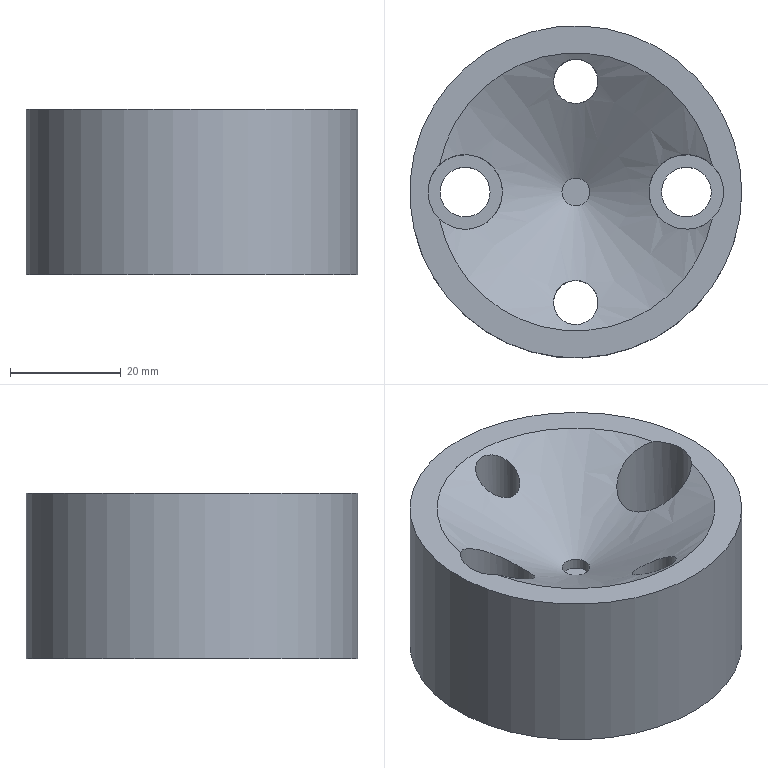Part | NX | features solid 2 | 1 solid | 14 faces | box 60 x 60 x 30 mm | volume 66301 mm3 | cylinder 8 | plane 5 | cone 1 | commonest cylinder face diameters 8 x2 9 x2 13.5 x2 5 x1 60 x1
STEP:
#1=CARTESIAN_POINT('',(335.,380.,0.));
#2=VERTEX_POINT('',#1);
#3=CARTESIAN_POINT('',(305.,380.,0.));
#4=DIRECTION('',(0.,0.,1.));
#5=DIRECTION('',(1.,0.,0.));
#6=AXIS2_PLACEMENT_3D('',#3,#4,#5);
#7=CIRCLE('',#6,30.);
#8=EDGE_CURVE('',#2,#2,#7,.T.);
#9=ORIENTED_EDGE('',*,*,#8,.T.);
#10=EDGE_LOOP('',(#9));
#11=FACE_BOUND('',#10,.T.);
#12=CARTESIAN_POINT('',(329.63,375.088,0.));
#13=VERTEX_POINT('',#12);
#14=CARTESIAN_POINT('',(329.63,384.912,0.));
#15=VERTEX_POINT('',#14);
#16=CARTESIAN_POINT('',(325.,380.,0.));
#17=DIRECTION('',(0.,0.,1.));
#18=DIRECTION('',(1.,0.,0.));
#19=AXIS2_PLACEMENT_3D('',#16,#17,#18);
#20=CIRCLE('',#19,6.75);
#21=EDGE_CURVE('',#13,#15,#20,.T.);
#22=ORIENTED_EDGE('',*,*,#21,.F.);
#23=CARTESIAN_POINT('',(280.37,375.088,0.));
#24=VERTEX_POINT('',#23);
#25=CARTESIAN_POINT('',(305.,380.,0.));
#26=DIRECTION('',(0.,0.,1.));
#27=DIRECTION('',(1.,0.,0.));
#28=AXIS2_PLACEMENT_3D('',#25,#26,#27);
#29=CIRCLE('',#28,25.115);
#30=EDGE_CURVE('',#13,#24,#29,.F.);
#31=ORIENTED_EDGE('',*,*,#30,.T.);
#32=CARTESIAN_POINT('',(280.37,384.912,0.));
#33=VERTEX_POINT('',#32);
#34=CARTESIAN_POINT('',(285.,380.,0.));
#35=DIRECTION('',(0.,0.,1.));
#36=DIRECTION('',(1.,0.,0.));
#37=AXIS2_PLACEMENT_3D('',#34,#35,#36);
#38=CIRCLE('',#37,6.75);
#39=EDGE_CURVE('',#33,#24,#38,.T.);
#40=ORIENTED_EDGE('',*,*,#39,.F.);
#41=CARTESIAN_POINT('',(305.,380.,0.));
#42=DIRECTION('',(0.,0.,1.));
#43=DIRECTION('',(1.,0.,0.));
#44=AXIS2_PLACEMENT_3D('',#41,#42,#43);
#45=CIRCLE('',#44,25.115);
#46=EDGE_CURVE('',#33,#15,#45,.F.);
#47=ORIENTED_EDGE('',*,*,#46,.T.);
#48=EDGE_LOOP('',(#22,#31,#40,#47));
#49=FACE_BOUND('',#48,.T.);
#50=CARTESIAN_POINT('',(305.,380.,0.));
#51=DIRECTION('',(0.,0.,1.));
#52=DIRECTION('',(1.,0.,0.));
#53=AXIS2_PLACEMENT_3D('',#50,#51,#52);
#54=PLANE('',#53);
#55=ADVANCED_FACE('',(#11,#49),#54,.T.);
#56=CARTESIAN_POINT('',(291.75,380.,-20.));
#57=VERTEX_POINT('',#56);
#58=CARTESIAN_POINT('',(285.,380.,-20.));
#59=DIRECTION('',(0.,0.,1.));
#60=DIRECTION('',(1.,0.,0.));
#61=AXIS2_PLACEMENT_3D('',#58,#59,#60);
#62=CIRCLE('',#61,6.75);
#63=EDGE_CURVE('',#57,#57,#62,.T.);
#64=ORIENTED_EDGE('',*,*,#63,.F.);
#65=EDGE_LOOP('',(#64));
#66=FACE_BOUND('',#65,.T.);
#67=ORIENTED_EDGE('',*,*,#39,.T.);
#68=CARTESIAN_POINT('',(280.37,375.088,0.));
#69=CARTESIAN_POINT('',(281.372,374.144,-0.4606));
#70=CARTESIAN_POINT('',(283.829,372.98,-1.636));
#71=CARTESIAN_POINT('',(287.691,373.437,-3.807));
#72=CARTESIAN_POINT('',(290.239,375.397,-5.595));
#73=CARTESIAN_POINT('',(291.504,377.82,-6.633));
#74=CARTESIAN_POINT('',(291.869,379.969,-6.955));
#75=CARTESIAN_POINT('',(291.521,382.134,-6.647));
#76=CARTESIAN_POINT('',(290.264,384.579,-5.614));
#77=CARTESIAN_POINT('',(287.696,386.564,-3.81));
#78=CARTESIAN_POINT('',(283.839,387.021,-1.641));
#79=CARTESIAN_POINT('',(281.375,385.859,-0.4617));
#80=CARTESIAN_POINT('',(280.37,384.912,0.));
#81=B_SPLINE_CURVE_WITH_KNOTS('',3,(#68,#69,#70,#71,#72,#73,#74,#75,#76,#77,#78,#79,#80),.UNSPECIFIED.,.F.,.F.,(4,1,1,1,1,1,1,1,1,1,4),(0.000000621,0.00429,0.008579,0.01287,0.01501,0.01716,0.0193,0.02145,0.02573,0.03002,0.03431),.UNSPECIFIED.);
#82=EDGE_CURVE('',#24,#33,#81,.T.);
#83=ORIENTED_EDGE('',*,*,#82,.T.);
#84=EDGE_LOOP('',(#67,#83));
#85=FACE_BOUND('',#84,.T.);
#86=CARTESIAN_POINT('',(285.,380.,0.));
#87=DIRECTION('',(0.,0.,-1.));
#88=DIRECTION('',(-1.,0.,0.));
#89=AXIS2_PLACEMENT_3D('',#86,#87,#88);
#90=CYLINDRICAL_SURFACE('',#89,6.75);
#91=ADVANCED_FACE('',(#66,#85),#90,.F.);
#92=CARTESIAN_POINT('',(331.75,380.,-20.));
#93=VERTEX_POINT('',#92);
#94=CARTESIAN_POINT('',(325.,380.,-20.));
#95=DIRECTION('',(0.,0.,1.));
#96=DIRECTION('',(1.,0.,0.));
#97=AXIS2_PLACEMENT_3D('',#94,#95,#96);
#98=CIRCLE('',#97,6.75);
#99=EDGE_CURVE('',#93,#93,#98,.T.);
#100=ORIENTED_EDGE('',*,*,#99,.F.);
#101=EDGE_LOOP('',(#100));
#102=FACE_BOUND('',#101,.T.);
#103=ORIENTED_EDGE('',*,*,#21,.T.);
#104=CARTESIAN_POINT('',(329.63,384.912,0.));
#105=CARTESIAN_POINT('',(328.628,385.856,-0.4606));
#106=CARTESIAN_POINT('',(326.171,387.02,-1.636));
#107=CARTESIAN_POINT('',(322.309,386.563,-3.807));
#108=CARTESIAN_POINT('',(319.761,384.603,-5.595));
#109=CARTESIAN_POINT('',(318.496,382.18,-6.633));
#110=CARTESIAN_POINT('',(318.131,380.031,-6.955));
#111=CARTESIAN_POINT('',(318.479,377.866,-6.647));
#112=CARTESIAN_POINT('',(319.736,375.421,-5.614));
#113=CARTESIAN_POINT('',(322.304,373.436,-3.81));
#114=CARTESIAN_POINT('',(326.161,372.979,-1.641));
#115=CARTESIAN_POINT('',(328.625,374.141,-0.4617));
#116=CARTESIAN_POINT('',(329.63,375.088,0.));
#117=B_SPLINE_CURVE_WITH_KNOTS('',3,(#104,#105,#106,#107,#108,#109,#110,#111,#112,#113,#114,#115,#116),.UNSPECIFIED.,.F.,.F.,(4,1,1,1,1,1,1,1,1,1,4),(0.000000621,0.00429,0.008579,0.01287,0.01501,0.01716,0.0193,0.02145,0.02573,0.03002,0.03431),.UNSPECIFIED.);
#118=EDGE_CURVE('',#15,#13,#117,.T.);
#119=ORIENTED_EDGE('',*,*,#118,.T.);
#120=EDGE_LOOP('',(#103,#119));
#121=FACE_BOUND('',#120,.T.);
#122=CARTESIAN_POINT('',(325.,380.,0.));
#123=DIRECTION('',(0.,0.,-1.));
#124=DIRECTION('',(-1.,0.,0.));
#125=AXIS2_PLACEMENT_3D('',#122,#123,#124);
#126=CYLINDRICAL_SURFACE('',#125,6.75);
#127=ADVANCED_FACE('',(#102,#121),#126,.F.);
#128=CARTESIAN_POINT('',(309.,360.,-30.));
#129=VERTEX_POINT('',#128);
#130=CARTESIAN_POINT('',(305.,360.,-30.));
#131=DIRECTION('',(0.,0.,1.));
#132=DIRECTION('',(1.,0.,0.));
#133=AXIS2_PLACEMENT_3D('',#130,#131,#132);
#134=CIRCLE('',#133,4.);
#135=EDGE_CURVE('',#129,#129,#134,.T.);
#136=ORIENTED_EDGE('',*,*,#135,.F.);
#137=EDGE_LOOP('',(#136));
#138=FACE_BOUND('',#137,.T.);
#139=CARTESIAN_POINT('',(302.043,357.307,-1.287));
#140=VERTEX_POINT('',#139);
#141=CARTESIAN_POINT('',(300.64,360.111,-2.741));
#142=CARTESIAN_POINT('',(301.661,357.063,-1.147));
#143=CARTESIAN_POINT('',(304.973,355.477,-0.3961));
#144=CARTESIAN_POINT('',(308.317,357.031,-1.131));
#145=CARTESIAN_POINT('',(309.36,360.084,-2.726));
#146=CARTESIAN_POINT('',(308.428,362.471,-4.197));
#147=CARTESIAN_POINT('',(306.716,363.738,-5.071));
#148=CARTESIAN_POINT('',(305.032,364.125,-5.353));
#149=CARTESIAN_POINT('',(303.333,363.762,-5.089));
#150=CARTESIAN_POINT('',(301.593,362.506,-4.219));
#151=CARTESIAN_POINT('',(300.64,360.111,-2.741));
#152=CARTESIAN_POINT('',(301.661,357.063,-1.147));
#153=CARTESIAN_POINT('',(304.973,355.477,-0.3961));
#154=B_SPLINE_CURVE_WITH_KNOTS('',3,(#141,#142,#143,#144,#145,#146,#147,#148,#149,#150,#151,#152,#153),.UNSPECIFIED.,.T.,.F.,(1,1,1,1,1,1,1,1,1,1,1,1,1,1,1,1,1),(-0.008433,-0.006746,-0.003373,0.,0.003373,0.006746,0.01012,0.01349,0.01518,0.01687,0.01855,0.02024,0.02361,0.02699,0.03036,0.03373,0.0371),.UNSPECIFIED.);
#155=EDGE_CURVE('',#140,#140,#154,.T.);
#156=ORIENTED_EDGE('',*,*,#155,.T.);
#157=EDGE_LOOP('',(#156));
#158=FACE_BOUND('',#157,.T.);
#159=CARTESIAN_POINT('',(305.,360.,0.));
#160=DIRECTION('',(0.,0.,-1.));
#161=DIRECTION('',(-1.,0.,0.));
#162=AXIS2_PLACEMENT_3D('',#159,#160,#161);
#163=CYLINDRICAL_SURFACE('',#162,4.);
#164=ADVANCED_FACE('',(#138,#158),#163,.F.);
#165=CARTESIAN_POINT('',(309.,400.,-30.));
#166=VERTEX_POINT('',#165);
#167=CARTESIAN_POINT('',(305.,400.,-30.));
#168=DIRECTION('',(0.,0.,1.));
#169=DIRECTION('',(1.,0.,0.));
#170=AXIS2_PLACEMENT_3D('',#167,#168,#169);
#171=CIRCLE('',#170,4.);
#172=EDGE_CURVE('',#166,#166,#171,.T.);
#173=ORIENTED_EDGE('',*,*,#172,.F.);
#174=EDGE_LOOP('',(#173));
#175=FACE_BOUND('',#174,.T.);
#176=CARTESIAN_POINT('',(302.431,396.934,-4.611));
#177=VERTEX_POINT('',#176);
#178=CARTESIAN_POINT('',(300.679,399.438,-2.999));
#179=CARTESIAN_POINT('',(301.874,397.138,-4.456));
#180=CARTESIAN_POINT('',(303.785,396.065,-5.214));
#181=CARTESIAN_POINT('',(305.52,395.91,-5.328));
#182=CARTESIAN_POINT('',(307.125,396.483,-4.914));
#183=CARTESIAN_POINT('',(308.661,397.902,-3.955));
#184=CARTESIAN_POINT('',(309.351,400.366,-2.475));
#185=CARTESIAN_POINT('',(307.972,403.332,-0.9555));
#186=CARTESIAN_POINT('',(304.43,404.487,-0.4129));
#187=CARTESIAN_POINT('',(301.365,402.54,-1.341));
#188=CARTESIAN_POINT('',(300.679,399.438,-2.999));
#189=CARTESIAN_POINT('',(301.874,397.138,-4.456));
#190=CARTESIAN_POINT('',(303.785,396.065,-5.214));
#191=B_SPLINE_CURVE_WITH_KNOTS('',3,(#178,#179,#180,#181,#182,#183,#184,#185,#186,#187,#188,#189,#190),.UNSPECIFIED.,.T.,.F.,(1,1,1,1,1,1,1,1,1,1,1,1,1,1,1,1,1),(-0.01012,-0.006749,-0.003375,0.,0.001687,0.003375,0.005062,0.006749,0.01012,0.0135,0.01687,0.02025,0.02362,0.027,0.02868,0.03037,0.03206),.UNSPECIFIED.);
#192=EDGE_CURVE('',#177,#177,#191,.T.);
#193=ORIENTED_EDGE('',*,*,#192,.T.);
#194=EDGE_LOOP('',(#193));
#195=FACE_BOUND('',#194,.T.);
#196=CARTESIAN_POINT('',(305.,400.,0.));
#197=DIRECTION('',(0.,0.,-1.));
#198=DIRECTION('',(-1.,0.,0.));
#199=AXIS2_PLACEMENT_3D('',#196,#197,#198);
#200=CYLINDRICAL_SURFACE('',#199,4.);
#201=ADVANCED_FACE('',(#175,#195),#200,.F.);
#202=ORIENTED_EDGE('',*,*,#135,.T.);
#203=EDGE_LOOP('',(#202));
#204=FACE_BOUND('',#203,.T.);
#205=CARTESIAN_POINT('',(289.5,380.,-30.));
#206=VERTEX_POINT('',#205);
#207=CARTESIAN_POINT('',(285.,380.,-30.));
#208=DIRECTION('',(0.,0.,1.));
#209=DIRECTION('',(1.,0.,0.));
#210=AXIS2_PLACEMENT_3D('',#207,#208,#209);
#211=CIRCLE('',#210,4.5);
#212=EDGE_CURVE('',#206,#206,#211,.T.);
#213=ORIENTED_EDGE('',*,*,#212,.T.);
#214=EDGE_LOOP('',(#213));
#215=FACE_BOUND('',#214,.T.);
#216=CARTESIAN_POINT('',(335.,380.,-30.));
#217=VERTEX_POINT('',#216);
#218=CARTESIAN_POINT('',(305.,380.,-30.));
#219=DIRECTION('',(0.,0.,1.));
#220=DIRECTION('',(1.,0.,0.));
#221=AXIS2_PLACEMENT_3D('',#218,#219,#220);
#222=CIRCLE('',#221,30.);
#223=EDGE_CURVE('',#217,#217,#222,.T.);
#224=ORIENTED_EDGE('',*,*,#223,.F.);
#225=EDGE_LOOP('',(#224));
#226=FACE_BOUND('',#225,.T.);
#227=CARTESIAN_POINT('',(329.5,380.,-30.));
#228=VERTEX_POINT('',#227);
#229=CARTESIAN_POINT('',(325.,380.,-30.));
#230=DIRECTION('',(0.,0.,1.));
#231=DIRECTION('',(1.,0.,0.));
#232=AXIS2_PLACEMENT_3D('',#229,#230,#231);
#233=CIRCLE('',#232,4.5);
#234=EDGE_CURVE('',#228,#228,#233,.T.);
#235=ORIENTED_EDGE('',*,*,#234,.T.);
#236=EDGE_LOOP('',(#235));
#237=FACE_BOUND('',#236,.T.);
#238=ORIENTED_EDGE('',*,*,#172,.T.);
#239=EDGE_LOOP('',(#238));
#240=FACE_BOUND('',#239,.T.);
#241=CARTESIAN_POINT('',(305.,380.,-30.));
#242=DIRECTION('',(0.,0.,1.));
#243=DIRECTION('',(1.,0.,0.));
#244=AXIS2_PLACEMENT_3D('',#241,#242,#243);
#245=PLANE('',#244);
#246=ADVANCED_FACE('',(#204,#215,#226,#237,#240),#245,.F.);
#247=ORIENTED_EDGE('',*,*,#99,.T.);
#248=EDGE_LOOP('',(#247));
#249=FACE_BOUND('',#248,.T.);
#250=CARTESIAN_POINT('',(329.5,380.,-20.));
#251=VERTEX_POINT('',#250);
#252=CARTESIAN_POINT('',(325.,380.,-20.));
#253=DIRECTION('',(0.,0.,1.));
#254=DIRECTION('',(1.,0.,0.));
#255=AXIS2_PLACEMENT_3D('',#252,#253,#254);
#256=CIRCLE('',#255,4.5);
#257=EDGE_CURVE('',#251,#251,#256,.T.);
#258=ORIENTED_EDGE('',*,*,#257,.F.);
#259=EDGE_LOOP('',(#258));
#260=FACE_BOUND('',#259,.T.);
#261=CARTESIAN_POINT('',(325.,380.,-20.));
#262=DIRECTION('',(0.,0.,1.));
#263=DIRECTION('',(1.,0.,0.));
#264=AXIS2_PLACEMENT_3D('',#261,#262,#263);
#265=PLANE('',#264);
#266=ADVANCED_FACE('',(#249,#260),#265,.T.);
#267=ORIENTED_EDGE('',*,*,#63,.T.);
#268=EDGE_LOOP('',(#267));
#269=FACE_BOUND('',#268,.T.);
#270=CARTESIAN_POINT('',(289.5,380.,-20.));
#271=VERTEX_POINT('',#270);
#272=CARTESIAN_POINT('',(285.,380.,-20.));
#273=DIRECTION('',(0.,0.,1.));
#274=DIRECTION('',(1.,0.,0.));
#275=AXIS2_PLACEMENT_3D('',#272,#273,#274);
#276=CIRCLE('',#275,4.5);
#277=EDGE_CURVE('',#271,#271,#276,.T.);
#278=ORIENTED_EDGE('',*,*,#277,.F.);
#279=EDGE_LOOP('',(#278));
#280=FACE_BOUND('',#279,.T.);
#281=CARTESIAN_POINT('',(285.,380.,-20.));
#282=DIRECTION('',(0.,0.,1.));
#283=DIRECTION('',(1.,0.,0.));
#284=AXIS2_PLACEMENT_3D('',#281,#282,#283);
#285=PLANE('',#284);
#286=ADVANCED_FACE('',(#269,#280),#285,.T.);
#287=ORIENTED_EDGE('',*,*,#8,.F.);
#288=EDGE_LOOP('',(#287));
#289=FACE_BOUND('',#288,.T.);
#290=ORIENTED_EDGE('',*,*,#223,.T.);
#291=EDGE_LOOP('',(#290));
#292=FACE_BOUND('',#291,.T.);
#293=CARTESIAN_POINT('',(305.,380.,0.));
#294=DIRECTION('',(0.,0.,-1.));
#295=DIRECTION('',(-1.,0.,0.));
#296=AXIS2_PLACEMENT_3D('',#293,#294,#295);
#297=CYLINDRICAL_SURFACE('',#296,30.);
#298=ADVANCED_FACE('',(#289,#292),#297,.T.);
#299=ORIENTED_EDGE('',*,*,#277,.T.);
#300=EDGE_LOOP('',(#299));
#301=FACE_BOUND('',#300,.T.);
#302=ORIENTED_EDGE('',*,*,#212,.F.);
#303=EDGE_LOOP('',(#302));
#304=FACE_BOUND('',#303,.T.);
#305=CARTESIAN_POINT('',(285.,380.,-20.));
#306=DIRECTION('',(0.,0.,-1.));
#307=DIRECTION('',(-1.,0.,0.));
#308=AXIS2_PLACEMENT_3D('',#305,#306,#307);
#309=CYLINDRICAL_SURFACE('',#308,4.5);
#310=ADVANCED_FACE('',(#301,#304),#309,.F.);
#311=ORIENTED_EDGE('',*,*,#257,.T.);
#312=EDGE_LOOP('',(#311));
#313=FACE_BOUND('',#312,.T.);
#314=ORIENTED_EDGE('',*,*,#234,.F.);
#315=EDGE_LOOP('',(#314));
#316=FACE_BOUND('',#315,.T.);
#317=CARTESIAN_POINT('',(325.,380.,-20.));
#318=DIRECTION('',(0.,0.,-1.));
#319=DIRECTION('',(-1.,0.,0.));
#320=AXIS2_PLACEMENT_3D('',#317,#318,#319);
#321=CYLINDRICAL_SURFACE('',#320,4.5);
#322=ADVANCED_FACE('',(#313,#316),#321,.F.);
#323=ORIENTED_EDGE('',*,*,#30,.F.);
#324=ORIENTED_EDGE('',*,*,#118,.F.);
#325=ORIENTED_EDGE('',*,*,#46,.F.);
#326=ORIENTED_EDGE('',*,*,#82,.F.);
#327=EDGE_LOOP('',(#323,#324,#325,#326));
#328=FACE_BOUND('',#327,.T.);
#329=ORIENTED_EDGE('',*,*,#155,.F.);
#330=EDGE_LOOP('',(#329));
#331=FACE_BOUND('',#330,.T.);
#332=ORIENTED_EDGE('',*,*,#192,.F.);
#333=EDGE_LOOP('',(#332));
#334=FACE_BOUND('',#333,.T.);
#335=CARTESIAN_POINT('',(307.5,380.,-13.057));
#336=VERTEX_POINT('',#335);
#337=CARTESIAN_POINT('',(305.,380.,-13.057));
#338=DIRECTION('',(0.,0.,1.));
#339=DIRECTION('',(1.,0.,0.));
#340=AXIS2_PLACEMENT_3D('',#337,#338,#339);
#341=CIRCLE('',#340,2.5);
#342=EDGE_CURVE('',#336,#336,#341,.F.);
#343=ORIENTED_EDGE('',*,*,#342,.T.);
#344=EDGE_LOOP('',(#343));
#345=FACE_BOUND('',#344,.T.);
#346=CARTESIAN_POINT('',(305.,380.,2.821));
#347=DIRECTION('',(0.,0.,1.));
#348=DIRECTION('',(1.,0.,0.));
#349=AXIS2_PLACEMENT_3D('',#346,#347,#348);
#350=CONICAL_SURFACE('',#349,30.,1.047);
#351=ADVANCED_FACE('',(#328,#331,#334,#345),#350,.F.);
#352=CARTESIAN_POINT('',(302.5,380.,-15.));
#353=VERTEX_POINT('',#352);
#354=CARTESIAN_POINT('',(305.,380.,-15.));
#355=DIRECTION('',(0.,0.,-1.));
#356=DIRECTION('',(-1.,0.,0.));
#357=AXIS2_PLACEMENT_3D('',#354,#355,#356);
#358=CIRCLE('',#357,2.5);
#359=EDGE_CURVE('',#353,#353,#358,.T.);
#360=ORIENTED_EDGE('',*,*,#359,.F.);
#361=EDGE_LOOP('',(#360));
#362=FACE_BOUND('',#361,.T.);
#363=CARTESIAN_POINT('',(305.,380.,-15.));
#364=DIRECTION('',(0.,0.,-1.));
#365=DIRECTION('',(-1.,0.,0.));
#366=AXIS2_PLACEMENT_3D('',#363,#364,#365);
#367=PLANE('',#366);
#368=ADVANCED_FACE('',(#362),#367,.F.);
#369=ORIENTED_EDGE('',*,*,#359,.T.);
#370=EDGE_LOOP('',(#369));
#371=FACE_BOUND('',#370,.T.);
#372=ORIENTED_EDGE('',*,*,#342,.F.);
#373=EDGE_LOOP('',(#372));
#374=FACE_BOUND('',#373,.T.);
#375=CARTESIAN_POINT('',(305.,380.,0.));
#376=DIRECTION('',(0.,0.,-1.));
#377=DIRECTION('',(-1.,0.,0.));
#378=AXIS2_PLACEMENT_3D('',#375,#376,#377);
#379=CYLINDRICAL_SURFACE('',#378,2.5);
#380=ADVANCED_FACE('',(#371,#374),#379,.F.);
#381=CLOSED_SHELL('',(#55,#91,#127,#164,#201,#246,#266,#286,#298,#310,#322,#351,#368,#380));
#382=MANIFOLD_SOLID_BREP('',#381);
#383=(LENGTH_UNIT()NAMED_UNIT(*)SI_UNIT(.MILLI.,.METRE.));
#384=UNCERTAINTY_MEASURE_WITH_UNIT(LENGTH_MEASURE(0.0508),#383,'','');
#385=(NAMED_UNIT(*)PLANE_ANGLE_UNIT()SI_UNIT($,.RADIAN.));
#386=(NAMED_UNIT(*)SI_UNIT($,.STERADIAN.)SOLID_ANGLE_UNIT());
#387=(GEOMETRIC_REPRESENTATION_CONTEXT(3)GLOBAL_UNCERTAINTY_ASSIGNED_CONTEXT((#384))GLOBAL_UNIT_ASSIGNED_CONTEXT((#383,#385,#386))REPRESENTATION_CONTEXT('',''));
#388=ADVANCED_BREP_SHAPE_REPRESENTATION('',(#382),#387);